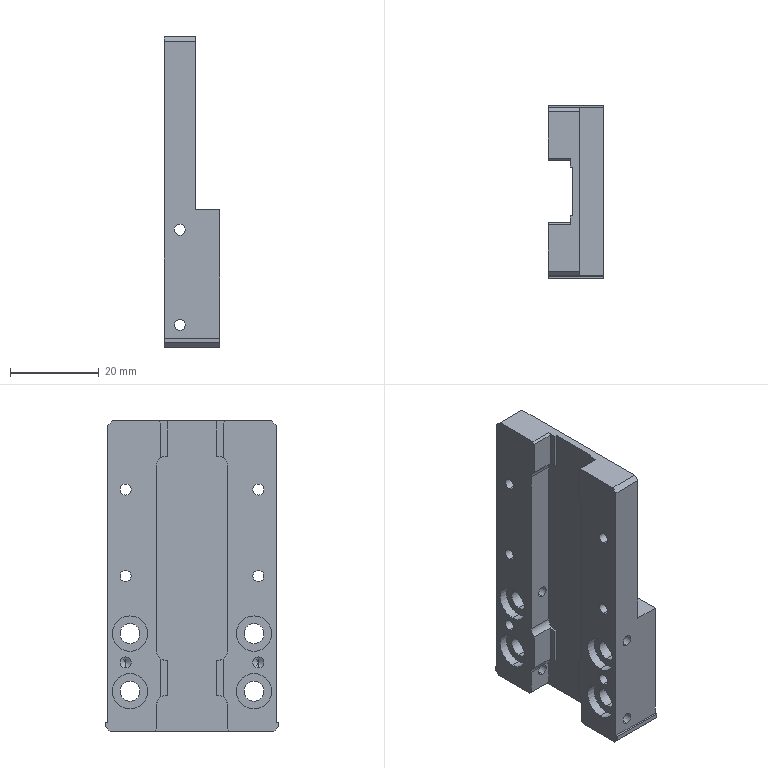Part | STEP file | Stopper bar limit plate | 1 solid | 94 faces | box 12.5 x 39 x 70 mm | volume 17639 mm3 | plane 48 | cylinder 42 | cone 4 | commonest cylinder face diameters 2.5 x20 4.5 x8 8 x8 4 x6